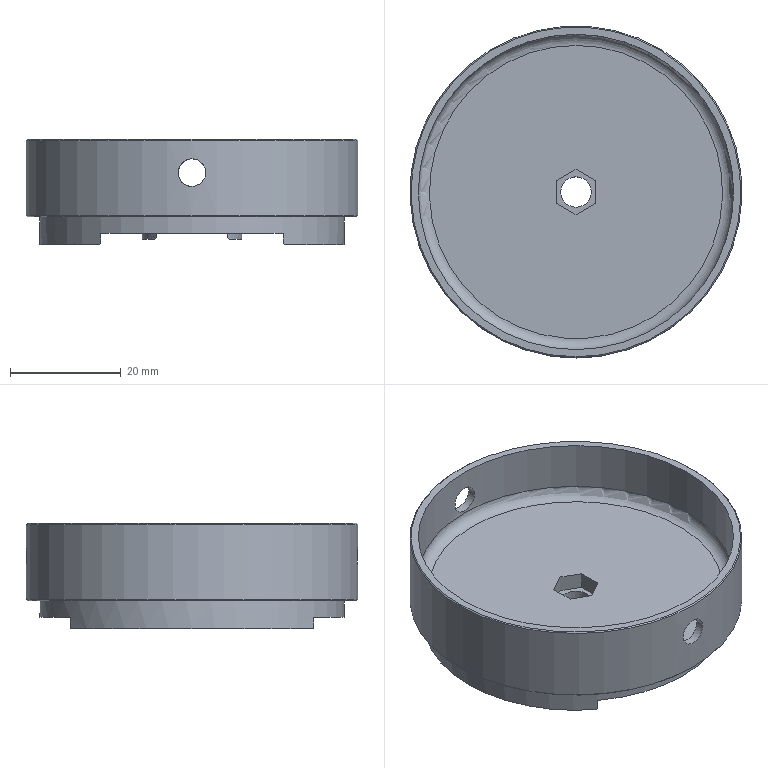NC program | NX | posted with a generic post | part box 60 x 60 x 19 mm
Lines 1 to 47 of 4306:
N10 G17 G21 G94 G90
(FLOOR_WALL , TOOL : D63)
N12 T01 M6
N14 G54
N16 G17 G0 G90 X-61.341 Y36.755 S1200 M3
N18 G43 Z30. H1
N20 Z3.
N22 G94 G1 Z0. F1250.
N24 X-57.814
N26 X57.816
N28 G2 X59.949 Y33.151 R67.666
N30 X61.035 Y31.109 R68.416
N32 X63.538 Y25.624 R68.136
N34 X68.5 Y1.582 R68.416
N36 G1 Y-1.588
N38 G2 X67.494 Y-11.8 R68.416
N40 G1 X-67.488
N42 X-70.532
N44 Z3.
N46 G0 Z30.
N48 M5
(DRILLING , TOOL : D8A45)
N50 T06 M6
N52 G54
N54 G17 G0 G90 X0. Y0. S5000 M3
N56 G43 Z30. H6
N58 G94 G81 G98 Z-1. F250. R3.
N60 G80
N62 G0 X0. Y0. Z30.
N64 M5
(DRILLING_COPY , TOOL : 5.5ZT)
N66 T15 M6
N68 G54
N70 G17 G0 G90 X0. Y0. S1000 M3
N72 G43 Z30. H15
N74 G94 G83 G98 Z-11.652 F150. Q3. R3.
N76 G80
N78 G0 X0. Y0. Z30.
N80 M5